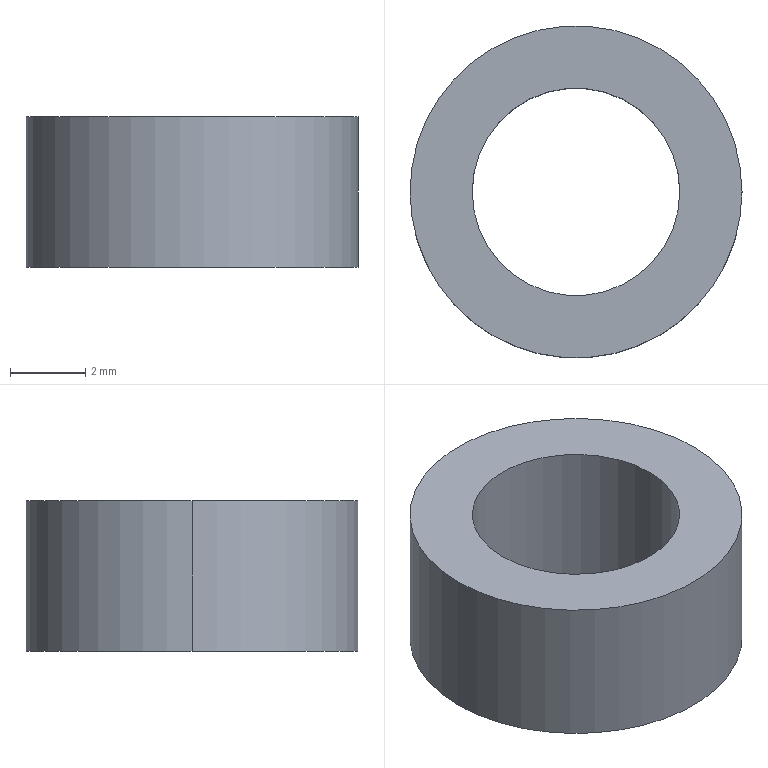Part | SolidWorks | features Extrusion 1 | 1 solid | 6 faces | box 8.8 x 8.8 x 4 mm | volume 148.252 mm3 | cylinder 4 | plane 2 | commonest cylinder face diameters 5.5 x2 8.8 x2
STEP:
#1=CARTESIAN_POINT('',(-2.75,0.,4.));
#2=VERTEX_POINT('',#1);
#3=CARTESIAN_POINT('',(2.75,0.,4.));
#4=VERTEX_POINT('',#3);
#5=CARTESIAN_POINT('',(0.,0.,4.));
#6=DIRECTION('',(0.,0.,1.));
#7=DIRECTION('',(1.,0.,0.));
#8=AXIS2_PLACEMENT_3D('',#5,#6,#7);
#9=CIRCLE('',#8,2.75);
#10=EDGE_CURVE('',#2,#4,#9,.T.);
#11=ORIENTED_EDGE('',*,*,#10,.T.);
#12=CARTESIAN_POINT('',(2.75,0.,0.));
#13=VERTEX_POINT('',#12);
#14=CARTESIAN_POINT('',(2.75,0.,4.));
#15=DIRECTION('',(0.,0.,-1.));
#16=VECTOR('',#15,1000.);
#17=LINE('',#14,#16);
#18=EDGE_CURVE('',#4,#13,#17,.T.);
#19=ORIENTED_EDGE('',*,*,#18,.T.);
#20=CARTESIAN_POINT('',(-2.75,0.,0.));
#21=VERTEX_POINT('',#20);
#22=CARTESIAN_POINT('',(0.,0.,0.));
#23=DIRECTION('',(0.,0.,1.));
#24=DIRECTION('',(1.,0.,0.));
#25=AXIS2_PLACEMENT_3D('',#22,#23,#24);
#26=CIRCLE('',#25,2.75);
#27=EDGE_CURVE('',#21,#13,#26,.T.);
#28=ORIENTED_EDGE('',*,*,#27,.F.);
#29=CARTESIAN_POINT('',(-2.75,0.,4.));
#30=DIRECTION('',(0.,0.,-1.));
#31=VECTOR('',#30,1000.);
#32=LINE('',#29,#31);
#33=EDGE_CURVE('',#2,#21,#32,.T.);
#34=ORIENTED_EDGE('',*,*,#33,.F.);
#35=EDGE_LOOP('',(#11,#19,#28,#34));
#36=FACE_OUTER_BOUND('',#35,.T.);
#37=CARTESIAN_POINT('',(0.,0.,4.));
#38=DIRECTION('',(0.,0.,-1.));
#39=DIRECTION('',(-1.,0.,0.));
#40=AXIS2_PLACEMENT_3D('',#37,#38,#39);
#41=CYLINDRICAL_SURFACE('',#40,2.75);
#42=ADVANCED_FACE('',(#36),#41,.F.);
#43=CARTESIAN_POINT('',(4.4,0.,4.));
#44=VERTEX_POINT('',#43);
#45=CARTESIAN_POINT('',(-4.4,0.,4.));
#46=VERTEX_POINT('',#45);
#47=CARTESIAN_POINT('',(0.,0.,4.));
#48=DIRECTION('',(0.,0.,1.));
#49=DIRECTION('',(1.,0.,0.));
#50=AXIS2_PLACEMENT_3D('',#47,#48,#49);
#51=CIRCLE('',#50,4.4);
#52=EDGE_CURVE('',#44,#46,#51,.T.);
#53=ORIENTED_EDGE('',*,*,#52,.F.);
#54=CARTESIAN_POINT('',(4.4,0.,0.));
#55=VERTEX_POINT('',#54);
#56=CARTESIAN_POINT('',(4.4,0.,4.));
#57=DIRECTION('',(0.,0.,-1.));
#58=VECTOR('',#57,1000.);
#59=LINE('',#56,#58);
#60=EDGE_CURVE('',#44,#55,#59,.T.);
#61=ORIENTED_EDGE('',*,*,#60,.T.);
#62=CARTESIAN_POINT('',(-4.4,0.,0.));
#63=VERTEX_POINT('',#62);
#64=CARTESIAN_POINT('',(0.,0.,0.));
#65=DIRECTION('',(0.,0.,1.));
#66=DIRECTION('',(1.,0.,0.));
#67=AXIS2_PLACEMENT_3D('',#64,#65,#66);
#68=CIRCLE('',#67,4.4);
#69=EDGE_CURVE('',#55,#63,#68,.T.);
#70=ORIENTED_EDGE('',*,*,#69,.T.);
#71=CARTESIAN_POINT('',(-4.4,0.,4.));
#72=DIRECTION('',(0.,0.,-1.));
#73=VECTOR('',#72,1000.);
#74=LINE('',#71,#73);
#75=EDGE_CURVE('',#46,#63,#74,.T.);
#76=ORIENTED_EDGE('',*,*,#75,.F.);
#77=EDGE_LOOP('',(#53,#61,#70,#76));
#78=FACE_OUTER_BOUND('',#77,.T.);
#79=CARTESIAN_POINT('',(0.,0.,4.));
#80=DIRECTION('',(0.,0.,-1.));
#81=DIRECTION('',(-1.,0.,0.));
#82=AXIS2_PLACEMENT_3D('',#79,#80,#81);
#83=CYLINDRICAL_SURFACE('',#82,4.4);
#84=ADVANCED_FACE('',(#78),#83,.T.);
#85=CARTESIAN_POINT('',(0.,0.,4.));
#86=DIRECTION('',(0.,0.,1.));
#87=DIRECTION('',(1.,0.,0.));
#88=AXIS2_PLACEMENT_3D('',#85,#86,#87);
#89=CIRCLE('',#88,4.4);
#90=EDGE_CURVE('',#46,#44,#89,.T.);
#91=ORIENTED_EDGE('',*,*,#90,.T.);
#92=ORIENTED_EDGE('',*,*,#52,.T.);
#93=EDGE_LOOP('',(#91,#92));
#94=FACE_OUTER_BOUND('',#93,.T.);
#95=ORIENTED_EDGE('',*,*,#10,.F.);
#96=CARTESIAN_POINT('',(0.,0.,4.));
#97=DIRECTION('',(0.,0.,1.));
#98=DIRECTION('',(1.,0.,0.));
#99=AXIS2_PLACEMENT_3D('',#96,#97,#98);
#100=CIRCLE('',#99,2.75);
#101=EDGE_CURVE('',#4,#2,#100,.T.);
#102=ORIENTED_EDGE('',*,*,#101,.F.);
#103=EDGE_LOOP('',(#95,#102));
#104=FACE_BOUND('',#103,.T.);
#105=CARTESIAN_POINT('',(0.,0.,4.));
#106=DIRECTION('',(0.,0.,1.));
#107=DIRECTION('',(1.,0.,0.));
#108=AXIS2_PLACEMENT_3D('',#105,#106,#107);
#109=PLANE('',#108);
#110=ADVANCED_FACE('',(#94,#104),#109,.T.);
#111=CARTESIAN_POINT('',(0.,0.,0.));
#112=DIRECTION('',(0.,0.,1.));
#113=DIRECTION('',(1.,0.,0.));
#114=AXIS2_PLACEMENT_3D('',#111,#112,#113);
#115=CIRCLE('',#114,4.4);
#116=EDGE_CURVE('',#63,#55,#115,.T.);
#117=ORIENTED_EDGE('',*,*,#116,.F.);
#118=ORIENTED_EDGE('',*,*,#69,.F.);
#119=EDGE_LOOP('',(#117,#118));
#120=FACE_OUTER_BOUND('',#119,.T.);
#121=ORIENTED_EDGE('',*,*,#27,.T.);
#122=CARTESIAN_POINT('',(0.,0.,0.));
#123=DIRECTION('',(0.,0.,1.));
#124=DIRECTION('',(1.,0.,0.));
#125=AXIS2_PLACEMENT_3D('',#122,#123,#124);
#126=CIRCLE('',#125,2.75);
#127=EDGE_CURVE('',#13,#21,#126,.T.);
#128=ORIENTED_EDGE('',*,*,#127,.T.);
#129=EDGE_LOOP('',(#121,#128));
#130=FACE_BOUND('',#129,.T.);
#131=CARTESIAN_POINT('',(0.,0.,0.));
#132=DIRECTION('',(0.,0.,1.));
#133=DIRECTION('',(1.,0.,0.));
#134=AXIS2_PLACEMENT_3D('',#131,#132,#133);
#135=PLANE('',#134);
#136=ADVANCED_FACE('',(#120,#130),#135,.F.);
#137=ORIENTED_EDGE('',*,*,#60,.F.);
#138=ORIENTED_EDGE('',*,*,#90,.F.);
#139=ORIENTED_EDGE('',*,*,#75,.T.);
#140=ORIENTED_EDGE('',*,*,#116,.T.);
#141=EDGE_LOOP('',(#137,#138,#139,#140));
#142=FACE_OUTER_BOUND('',#141,.T.);
#143=CARTESIAN_POINT('',(0.,0.,4.));
#144=DIRECTION('',(0.,0.,-1.));
#145=DIRECTION('',(-1.,0.,0.));
#146=AXIS2_PLACEMENT_3D('',#143,#144,#145);
#147=CYLINDRICAL_SURFACE('',#146,4.4);
#148=ADVANCED_FACE('',(#142),#147,.T.);
#149=ORIENTED_EDGE('',*,*,#18,.F.);
#150=ORIENTED_EDGE('',*,*,#101,.T.);
#151=ORIENTED_EDGE('',*,*,#33,.T.);
#152=ORIENTED_EDGE('',*,*,#127,.F.);
#153=EDGE_LOOP('',(#149,#150,#151,#152));
#154=FACE_OUTER_BOUND('',#153,.T.);
#155=CARTESIAN_POINT('',(0.,0.,4.));
#156=DIRECTION('',(0.,0.,-1.));
#157=DIRECTION('',(-1.,0.,0.));
#158=AXIS2_PLACEMENT_3D('',#155,#156,#157);
#159=CYLINDRICAL_SURFACE('',#158,2.75);
#160=ADVANCED_FACE('',(#154),#159,.F.);
#161=CLOSED_SHELL('',(#42,#84,#110,#136,#148,#160));
#162=MANIFOLD_SOLID_BREP('',#161);
#163=CARTESIAN_POINT('',(0.,0.,0.));
#164=DIRECTION('',(0.,0.,1.));
#165=DIRECTION('',(1.,0.,0.));
#166=AXIS2_PLACEMENT_3D('',#163,#164,#165);
#167=(LENGTH_UNIT()NAMED_UNIT(*)SI_UNIT(.MILLI.,.METRE.));
#168=UNCERTAINTY_MEASURE_WITH_UNIT(LENGTH_MEASURE(0.00001),#167,'','');
#169=(NAMED_UNIT(*)PLANE_ANGLE_UNIT()SI_UNIT($,.RADIAN.));
#170=(NAMED_UNIT(*)SI_UNIT($,.STERADIAN.)SOLID_ANGLE_UNIT());
#171=(GEOMETRIC_REPRESENTATION_CONTEXT(3)GLOBAL_UNCERTAINTY_ASSIGNED_CONTEXT((#168))GLOBAL_UNIT_ASSIGNED_CONTEXT((#167,#169,#170))REPRESENTATION_CONTEXT('',''));
#172=ADVANCED_BREP_SHAPE_REPRESENTATION('',(#162,#166),#171);